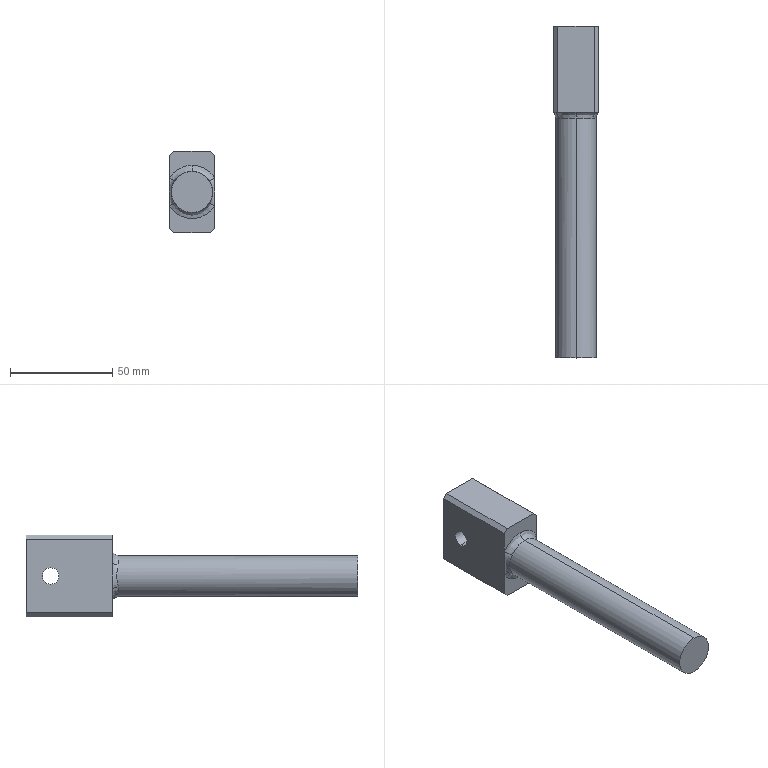Part | STEP file | 1 solid | 21 faces | box 22 x 162 x 40 mm | volume 73328 mm3 | plane 12 | spline 5 | cylinder 4 | commonest cylinder face diameters 8 x2 20 x2